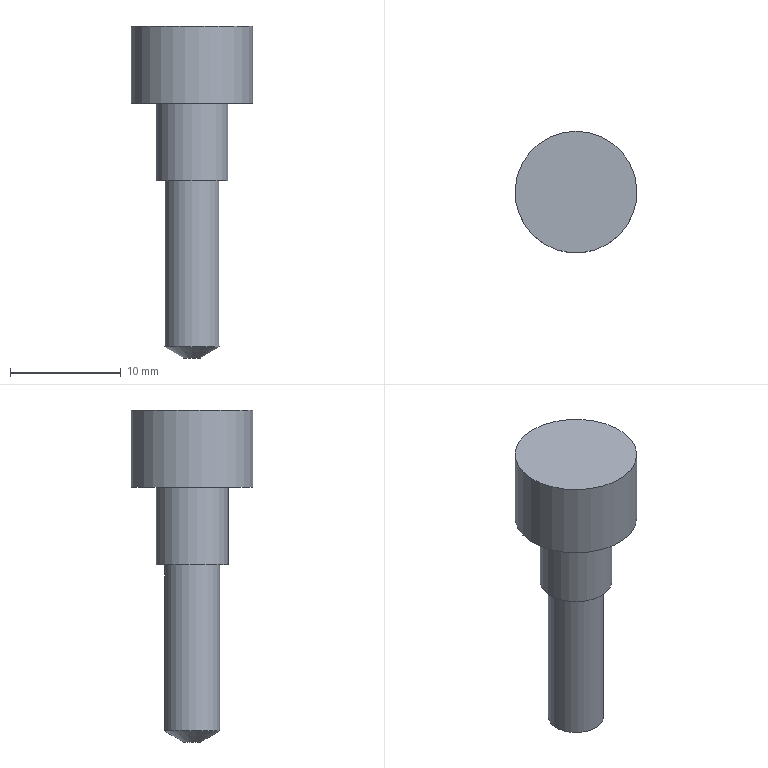Part | STEP file | solid 129 | 1 solid | 8 faces | box 11 x 11 x 30 mm | volume 1201 mm3 | plane 4 | cylinder 3 | cone 1 | commonest cylinder face diameters 5 x1 6.5 x1 11 x1